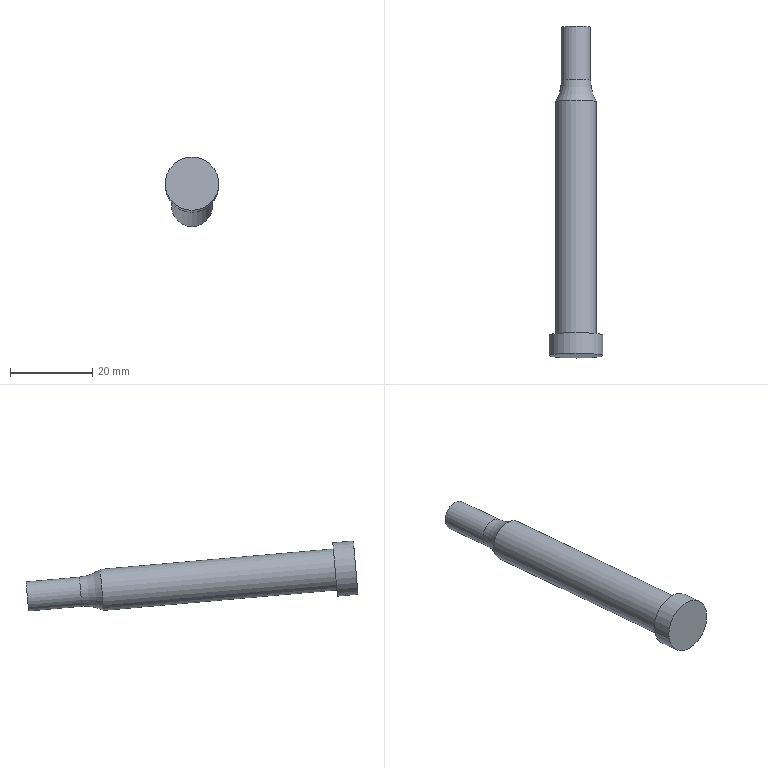Part | NX | features SPAS-C 10-80-7.100 2 | 1 solid | 7 faces | box 13 x 80.571 x 16.984 mm | volume 5907 mm3 | plane 3 | cylinder 3 | torus 1 | commonest cylinder face diameters 7.1 x1 10 x1 13 x1
STEP:
#1=CARTESIAN_POINT('',(169.288,-39.687,-28.235));
#2=VERTEX_POINT('',#1);
#3=CARTESIAN_POINT('',(169.288,-39.996,-31.771));
#4=DIRECTION('',(0.,-0.9962,0.08716));
#5=DIRECTION('',(0.,0.08716,0.9962));
#6=AXIS2_PLACEMENT_3D('',#3,#4,#5);
#7=CIRCLE('',#6,3.55);
#8=EDGE_CURVE('',#2,#2,#7,.T.);
#9=ORIENTED_EDGE('',*,*,#8,.F.);
#10=EDGE_LOOP('',(#9));
#11=FACE_BOUND('',#10,.T.);
#12=CARTESIAN_POINT('',(169.288,-39.996,-31.771));
#13=DIRECTION('',(0.,0.9962,-0.08716));
#14=DIRECTION('',(0.,-0.08716,-0.9962));
#15=AXIS2_PLACEMENT_3D('',#12,#13,#14);
#16=PLANE('',#15);
#17=ADVANCED_FACE('',(#11),#16,.T.);
#18=CARTESIAN_POINT('',(169.288,-52.637,-27.102));
#19=VERTEX_POINT('',#18);
#20=CARTESIAN_POINT('',(169.288,-52.947,-30.638));
#21=DIRECTION('',(0.,-0.9962,0.08716));
#22=DIRECTION('',(0.,0.08716,0.9962));
#23=AXIS2_PLACEMENT_3D('',#20,#21,#22);
#24=CIRCLE('',#23,3.55);
#25=EDGE_CURVE('',#19,#19,#24,.F.);
#26=ORIENTED_EDGE('',*,*,#25,.T.);
#27=EDGE_LOOP('',(#26));
#28=FACE_BOUND('',#27,.T.);
#29=ORIENTED_EDGE('',*,*,#8,.T.);
#30=EDGE_LOOP('',(#29));
#31=FACE_BOUND('',#30,.T.);
#32=CARTESIAN_POINT('',(169.288,-39.996,-31.771));
#33=DIRECTION('',(0.,-0.9962,0.08716));
#34=DIRECTION('',(0.,0.08716,0.9962));
#35=AXIS2_PLACEMENT_3D('',#32,#33,#34);
#36=CYLINDRICAL_SURFACE('',#35,3.55);
#37=ADVANCED_FACE('',(#28,#31),#36,.T.);
#38=CARTESIAN_POINT('',(169.288,-114.275,-20.253));
#39=VERTEX_POINT('',#38);
#40=CARTESIAN_POINT('',(169.288,-114.711,-25.234));
#41=DIRECTION('',(0.,0.9962,-0.08716));
#42=DIRECTION('',(0.,0.08716,0.9962));
#43=AXIS2_PLACEMENT_3D('',#40,#41,#42);
#44=CIRCLE('',#43,5.);
#45=EDGE_CURVE('',#39,#39,#44,.F.);
#46=ORIENTED_EDGE('',*,*,#45,.F.);
#47=EDGE_LOOP('',(#46));
#48=FACE_BOUND('',#47,.T.);
#49=CARTESIAN_POINT('',(169.288,-57.678,-25.205));
#50=VERTEX_POINT('',#49);
#51=CARTESIAN_POINT('',(169.288,-58.113,-30.186));
#52=DIRECTION('',(0.,-0.9962,0.08716));
#53=DIRECTION('',(0.,0.08716,0.9962));
#54=AXIS2_PLACEMENT_3D('',#51,#52,#53);
#55=CIRCLE('',#54,5.);
#56=EDGE_CURVE('',#50,#50,#55,.T.);
#57=ORIENTED_EDGE('',*,*,#56,.T.);
#58=EDGE_LOOP('',(#57));
#59=FACE_BOUND('',#58,.T.);
#60=CARTESIAN_POINT('',(169.288,-58.113,-30.186));
#61=DIRECTION('',(0.,-0.9962,0.08716));
#62=DIRECTION('',(0.,0.08716,0.9962));
#63=AXIS2_PLACEMENT_3D('',#60,#61,#62);
#64=CYLINDRICAL_SURFACE('',#63,5.);
#65=ADVANCED_FACE('',(#48,#59),#64,.T.);
#66=CARTESIAN_POINT('',(169.288,-120.258,-31.274));
#67=VERTEX_POINT('',#66);
#68=CARTESIAN_POINT('',(169.288,-119.692,-24.799));
#69=DIRECTION('',(0.,-0.9962,0.08716));
#70=DIRECTION('',(0.,-0.08716,-0.9962));
#71=AXIS2_PLACEMENT_3D('',#68,#69,#70);
#72=CIRCLE('',#71,6.5);
#73=EDGE_CURVE('',#67,#67,#72,.F.);
#74=ORIENTED_EDGE('',*,*,#73,.F.);
#75=EDGE_LOOP('',(#74));
#76=FACE_BOUND('',#75,.T.);
#77=CARTESIAN_POINT('',(169.288,-119.692,-24.799));
#78=DIRECTION('',(0.,-0.9962,0.08716));
#79=DIRECTION('',(0.,0.08716,0.9962));
#80=AXIS2_PLACEMENT_3D('',#77,#78,#79);
#81=PLANE('',#80);
#82=ADVANCED_FACE('',(#76),#81,.T.);
#83=ORIENTED_EDGE('',*,*,#45,.T.);
#84=EDGE_LOOP('',(#83));
#85=FACE_BOUND('',#84,.T.);
#86=CARTESIAN_POINT('',(169.288,-114.144,-18.759));
#87=VERTEX_POINT('',#86);
#88=CARTESIAN_POINT('',(169.288,-114.711,-25.234));
#89=DIRECTION('',(0.,0.9962,-0.08716));
#90=DIRECTION('',(0.,0.08716,0.9962));
#91=AXIS2_PLACEMENT_3D('',#88,#89,#90);
#92=CIRCLE('',#91,6.5);
#93=EDGE_CURVE('',#87,#87,#92,.F.);
#94=ORIENTED_EDGE('',*,*,#93,.F.);
#95=EDGE_LOOP('',(#94));
#96=FACE_BOUND('',#95,.T.);
#97=CARTESIAN_POINT('',(169.288,-114.711,-25.234));
#98=DIRECTION('',(0.,0.9962,-0.08716));
#99=DIRECTION('',(0.,-0.08716,-0.9962));
#100=AXIS2_PLACEMENT_3D('',#97,#98,#99);
#101=PLANE('',#100);
#102=ADVANCED_FACE('',(#85,#96),#101,.T.);
#103=ORIENTED_EDGE('',*,*,#73,.T.);
#104=EDGE_LOOP('',(#103));
#105=FACE_BOUND('',#104,.T.);
#106=ORIENTED_EDGE('',*,*,#93,.T.);
#107=EDGE_LOOP('',(#106));
#108=FACE_BOUND('',#107,.T.);
#109=CARTESIAN_POINT('',(169.288,-114.711,-25.234));
#110=DIRECTION('',(0.,-0.9962,0.08716));
#111=DIRECTION('',(0.,0.08716,0.9962));
#112=AXIS2_PLACEMENT_3D('',#109,#110,#111);
#113=CYLINDRICAL_SURFACE('',#112,6.5);
#114=ADVANCED_FACE('',(#105,#108),#113,.T.);
#115=ORIENTED_EDGE('',*,*,#25,.F.);
#116=EDGE_LOOP('',(#115));
#117=FACE_BOUND('',#116,.T.);
#118=ORIENTED_EDGE('',*,*,#56,.F.);
#119=EDGE_LOOP('',(#118));
#120=FACE_BOUND('',#119,.T.);
#121=CARTESIAN_POINT('',(169.288,-52.947,-30.638));
#122=DIRECTION('',(0.,-0.9962,0.08716));
#123=DIRECTION('',(0.,0.08716,0.9962));
#124=AXIS2_PLACEMENT_3D('',#121,#122,#123);
#125=TOROIDAL_SURFACE('',#124,13.55,10.);
#126=ADVANCED_FACE('',(#117,#120),#125,.F.);
#127=CLOSED_SHELL('',(#17,#37,#65,#82,#102,#114,#126));
#128=MANIFOLD_SOLID_BREP('',#127);
#129=(LENGTH_UNIT()NAMED_UNIT(*)SI_UNIT(.MILLI.,.METRE.));
#130=UNCERTAINTY_MEASURE_WITH_UNIT(LENGTH_MEASURE(0.00001),#129,'','');
#131=(NAMED_UNIT(*)PLANE_ANGLE_UNIT()SI_UNIT($,.RADIAN.));
#132=(NAMED_UNIT(*)SI_UNIT($,.STERADIAN.)SOLID_ANGLE_UNIT());
#133=(GEOMETRIC_REPRESENTATION_CONTEXT(3)GLOBAL_UNCERTAINTY_ASSIGNED_CONTEXT((#130))GLOBAL_UNIT_ASSIGNED_CONTEXT((#129,#131,#132))REPRESENTATION_CONTEXT('',''));
#134=ADVANCED_BREP_SHAPE_REPRESENTATION('',(#128),#133);